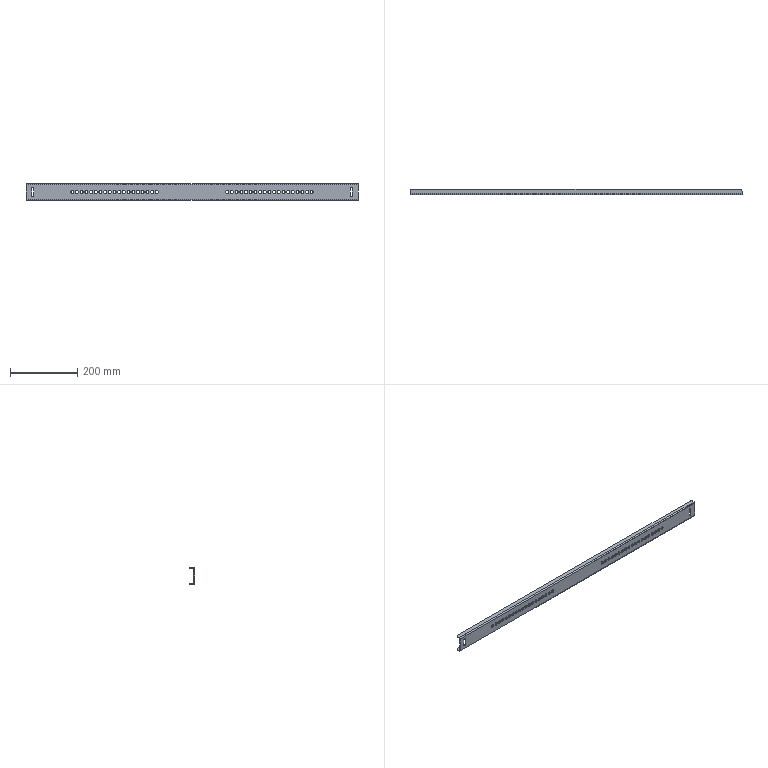Part | SolidWorks | features ICE 2, EdgeFlange 1, Fillet 1, FlatPattern 1, HoleWzd 1, LPattern 1, MirrorPattern 1, SMBaseFlange 1, SheetMetal 1 | 1 solid | 112 faces | box 990 x 15 x 50 mm | volume 140813 mm3 | cylinder 90 | plane 22 | commonest cylinder face diameters 9.2 x76 7 x6 10 x4 2.54 x2 6.54 x2